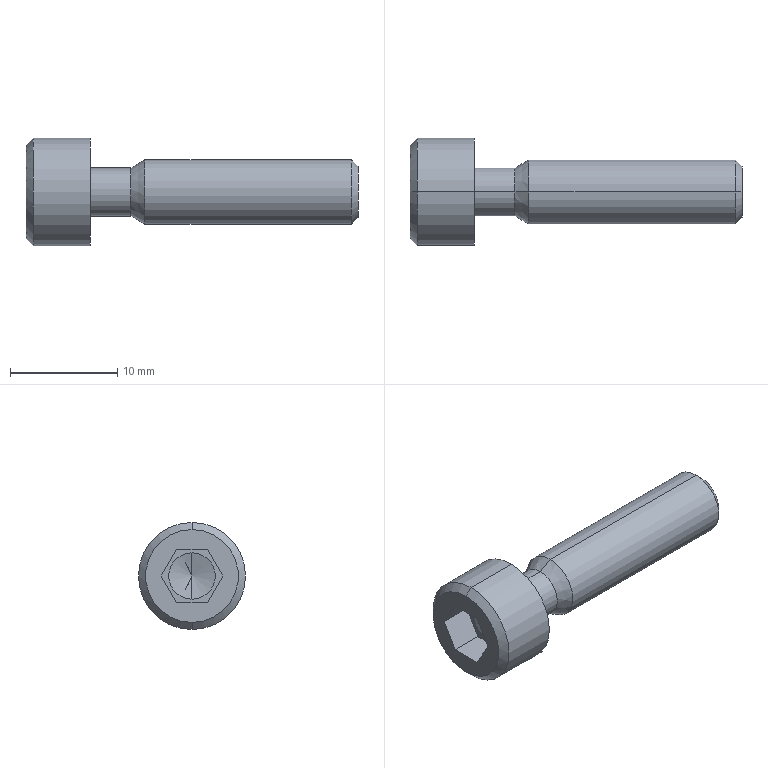Part | STEP file | 0244_Z_019_SCBZ6-25_1 | 1 solid | 24 faces | box 31 x 10 x 10 mm | volume 1045 mm3 | plane 10 | cone 8 | cylinder 6 | commonest cylinder face diameters 4.5 x2 6 x2 10 x2
STEP:
#1=CARTESIAN_POINT('',(0.,0.,0.));
#2=DIRECTION('',(0.,0.,1.));
#3=DIRECTION('',(1.,0.,0.));
#4=AXIS2_PLACEMENT_3D('',#1,#2,#3);
#5=CARTESIAN_POINT('',(5.1,0.,-3.));
#6=VERTEX_POINT('',#5);
#7=CARTESIAN_POINT('',(5.1,0.,3.));
#8=VERTEX_POINT('',#7);
#9=CARTESIAN_POINT('',(5.1,0.,0.));
#10=DIRECTION('',(1.,0.,0.));
#11=DIRECTION('',(0.,0.,-1.));
#12=AXIS2_PLACEMENT_3D('',#9,#10,#11);
#13=CIRCLE('',#12,3.);
#14=CARTESIAN_POINT('',(14.743,0.,0.));
#15=DIRECTION('',(1.,0.,0.));
#16=DIRECTION('',(0.,0.,-1.));
#17=AXIS2_PLACEMENT_3D('',#14,#15,#16);
#18=CYLINDRICAL_SURFACE('',#17,3.);
#19=CARTESIAN_POINT('',(0.,-9.643));
#20=DIRECTION('',(1.,0.));
#21=VECTOR('',#20,1.);
#22=LINE('',#19,#21);
#23=(GEOMETRIC_REPRESENTATION_CONTEXT(2)PARAMETRIC_REPRESENTATION_CONTEXT()REPRESENTATION_CONTEXT('',''));
#24=DEFINITIONAL_REPRESENTATION('',(#22),#23);
#25=PCURVE('',#18,#24);
#26=CARTESIAN_POINT('',(5.1,0.,0.));
#27=DIRECTION('',(1.,0.,0.));
#28=DIRECTION('',(0.,0.,-1.));
#29=AXIS2_PLACEMENT_3D('',#26,#27,#28);
#30=CONICAL_SURFACE('',#29,3.,0.5236);
#31=CARTESIAN_POINT('',(0.,0.));
#32=DIRECTION('',(1.,0.));
#33=VECTOR('',#32,1.);
#34=LINE('',#31,#33);
#35=(GEOMETRIC_REPRESENTATION_CONTEXT(2)PARAMETRIC_REPRESENTATION_CONTEXT()REPRESENTATION_CONTEXT('',''));
#36=DEFINITIONAL_REPRESENTATION('',(#34),#35);
#37=PCURVE('',#30,#36);
#38=SURFACE_CURVE('',#13,(#25,#37),.PCURVE_S1.);
#39=EDGE_CURVE('',#6,#8,#38,.T.);
#40=ORIENTED_EDGE('',*,*,#39,.T.);
#41=CARTESIAN_POINT('',(24.387,0.,3.));
#42=VERTEX_POINT('',#41);
#43=CARTESIAN_POINT('',(14.743,0.,3.));
#44=DIRECTION('',(1.,0.,0.));
#45=VECTOR('',#44,1.);
#46=LINE('',#43,#45);
#47=CARTESIAN_POINT('',(3.142,0.));
#48=DIRECTION('',(0.,1.));
#49=VECTOR('',#48,1.);
#50=LINE('',#47,#49);
#51=(GEOMETRIC_REPRESENTATION_CONTEXT(2)PARAMETRIC_REPRESENTATION_CONTEXT()REPRESENTATION_CONTEXT('',''));
#52=DEFINITIONAL_REPRESENTATION('',(#50),#51);
#53=PCURVE('',#18,#52);
#54=CARTESIAN_POINT('',(14.743,0.,0.));
#55=DIRECTION('',(1.,0.,0.));
#56=DIRECTION('',(0.,0.,-1.));
#57=AXIS2_PLACEMENT_3D('',#54,#55,#56);
#58=CYLINDRICAL_SURFACE('',#57,3.);
#59=CARTESIAN_POINT('',(3.142,0.));
#60=DIRECTION('',(0.,1.));
#61=VECTOR('',#60,1.);
#62=LINE('',#59,#61);
#63=(GEOMETRIC_REPRESENTATION_CONTEXT(2)PARAMETRIC_REPRESENTATION_CONTEXT()REPRESENTATION_CONTEXT('',''));
#64=DEFINITIONAL_REPRESENTATION('',(#62),#63);
#65=PCURVE('',#58,#64);
#66=SURFACE_CURVE('',#46,(#53,#65),.PCURVE_S1.);
#67=EDGE_CURVE('',#8,#42,#66,.T.);
#68=ORIENTED_EDGE('',*,*,#67,.T.);
#69=CARTESIAN_POINT('',(24.387,0.,-3.));
#70=VERTEX_POINT('',#69);
#71=CARTESIAN_POINT('',(24.387,0.,0.));
#72=DIRECTION('',(-1.,0.,0.));
#73=DIRECTION('',(0.,0.,-1.));
#74=AXIS2_PLACEMENT_3D('',#71,#72,#73);
#75=CIRCLE('',#74,3.);
#76=CARTESIAN_POINT('',(6.283,9.643));
#77=DIRECTION('',(-1.,0.));
#78=VECTOR('',#77,1.);
#79=LINE('',#76,#78);
#80=(GEOMETRIC_REPRESENTATION_CONTEXT(2)PARAMETRIC_REPRESENTATION_CONTEXT()REPRESENTATION_CONTEXT('',''));
#81=DEFINITIONAL_REPRESENTATION('',(#79),#80);
#82=PCURVE('',#18,#81);
#83=CARTESIAN_POINT('',(24.386,0.,0.));
#84=DIRECTION('',(-1.,0.,0.));
#85=DIRECTION('',(0.,0.,1.));
#86=AXIS2_PLACEMENT_3D('',#83,#84,#85);
#87=CONICAL_SURFACE('',#86,3.,0.7854);
#88=CARTESIAN_POINT('',(-3.142,0.));
#89=DIRECTION('',(1.,0.));
#90=VECTOR('',#89,1.);
#91=LINE('',#88,#90);
#92=(GEOMETRIC_REPRESENTATION_CONTEXT(2)PARAMETRIC_REPRESENTATION_CONTEXT()REPRESENTATION_CONTEXT('',''));
#93=DEFINITIONAL_REPRESENTATION('',(#91),#92);
#94=PCURVE('',#87,#93);
#95=SURFACE_CURVE('',#75,(#82,#94),.PCURVE_S1.);
#96=EDGE_CURVE('',#42,#70,#95,.T.);
#97=ORIENTED_EDGE('',*,*,#96,.T.);
#98=CARTESIAN_POINT('',(14.743,0.,-3.));
#99=DIRECTION('',(1.,0.,0.));
#100=VECTOR('',#99,1.);
#101=LINE('',#98,#100);
#102=CARTESIAN_POINT('',(0.,0.));
#103=DIRECTION('',(0.,1.));
#104=VECTOR('',#103,1.);
#105=LINE('',#102,#104);
#106=(GEOMETRIC_REPRESENTATION_CONTEXT(2)PARAMETRIC_REPRESENTATION_CONTEXT()REPRESENTATION_CONTEXT('',''));
#107=DEFINITIONAL_REPRESENTATION('',(#105),#106);
#108=PCURVE('',#18,#107);
#109=CARTESIAN_POINT('',(6.283,0.));
#110=DIRECTION('',(0.,1.));
#111=VECTOR('',#110,1.);
#112=LINE('',#109,#111);
#113=(GEOMETRIC_REPRESENTATION_CONTEXT(2)PARAMETRIC_REPRESENTATION_CONTEXT()REPRESENTATION_CONTEXT('',''));
#114=DEFINITIONAL_REPRESENTATION('',(#112),#113);
#115=PCURVE('',#58,#114);
#116=SURFACE_CURVE('',#101,(#108,#115),.PCURVE_S1.);
#117=EDGE_CURVE('',#6,#70,#116,.T.);
#118=ORIENTED_EDGE('',*,*,#117,.F.);
#119=EDGE_LOOP('',(#40,#68,#97,#118));
#120=FACE_BOUND('',#119,.T.);
#121=ADVANCED_FACE('',(#120),#18,.T.);
#122=CARTESIAN_POINT('',(3.801,0.,-2.25));
#123=VERTEX_POINT('',#122);
#124=CARTESIAN_POINT('',(3.801,0.,2.25));
#125=VERTEX_POINT('',#124);
#126=CARTESIAN_POINT('',(3.801,0.,0.));
#127=DIRECTION('',(1.,0.,0.));
#128=DIRECTION('',(0.,1.,0.));
#129=AXIS2_PLACEMENT_3D('',#126,#127,#128);
#130=CIRCLE('',#129,2.25);
#131=CARTESIAN_POINT('',(-4.712,-1.299));
#132=DIRECTION('',(1.,0.));
#133=VECTOR('',#132,1.);
#134=LINE('',#131,#133);
#135=(GEOMETRIC_REPRESENTATION_CONTEXT(2)PARAMETRIC_REPRESENTATION_CONTEXT()REPRESENTATION_CONTEXT('',''));
#136=DEFINITIONAL_REPRESENTATION('',(#134),#135);
#137=PCURVE('',#30,#136);
#138=CARTESIAN_POINT('',(1.9,0.,0.));
#139=DIRECTION('',(1.,0.,0.));
#140=DIRECTION('',(0.,0.,-1.));
#141=AXIS2_PLACEMENT_3D('',#138,#139,#140);
#142=CYLINDRICAL_SURFACE('',#141,2.25);
#143=CARTESIAN_POINT('',(-4.712,1.9));
#144=DIRECTION('',(1.,0.));
#145=VECTOR('',#144,1.);
#146=LINE('',#143,#145);
#147=(GEOMETRIC_REPRESENTATION_CONTEXT(2)PARAMETRIC_REPRESENTATION_CONTEXT()REPRESENTATION_CONTEXT('',''));
#148=DEFINITIONAL_REPRESENTATION('',(#146),#147);
#149=PCURVE('',#142,#148);
#150=SURFACE_CURVE('',#130,(#137,#149),.PCURVE_S1.);
#151=EDGE_CURVE('',#123,#125,#150,.T.);
#152=ORIENTED_EDGE('',*,*,#151,.T.);
#153=CARTESIAN_POINT('',(5.1,0.,3.));
#154=DIRECTION('',(0.866,0.,0.5));
#155=VECTOR('',#154,1.);
#156=LINE('',#153,#155);
#157=CARTESIAN_POINT('',(3.142,0.));
#158=DIRECTION('',(0.,1.));
#159=VECTOR('',#158,1.);
#160=LINE('',#157,#159);
#161=(GEOMETRIC_REPRESENTATION_CONTEXT(2)PARAMETRIC_REPRESENTATION_CONTEXT()REPRESENTATION_CONTEXT('',''));
#162=DEFINITIONAL_REPRESENTATION('',(#160),#161);
#163=PCURVE('',#30,#162);
#164=CARTESIAN_POINT('',(5.1,0.,0.));
#165=DIRECTION('',(1.,0.,0.));
#166=DIRECTION('',(0.,0.,-1.));
#167=AXIS2_PLACEMENT_3D('',#164,#165,#166);
#168=CONICAL_SURFACE('',#167,3.,0.5236);
#169=CARTESIAN_POINT('',(3.142,0.));
#170=DIRECTION('',(0.,1.));
#171=VECTOR('',#170,1.);
#172=LINE('',#169,#171);
#173=(GEOMETRIC_REPRESENTATION_CONTEXT(2)PARAMETRIC_REPRESENTATION_CONTEXT()REPRESENTATION_CONTEXT('',''));
#174=DEFINITIONAL_REPRESENTATION('',(#172),#173);
#175=PCURVE('',#168,#174);
#176=SURFACE_CURVE('',#156,(#163,#175),.PCURVE_S1.);
#177=EDGE_CURVE('',#125,#8,#176,.T.);
#178=ORIENTED_EDGE('',*,*,#177,.T.);
#179=ORIENTED_EDGE('',*,*,#39,.F.);
#180=CARTESIAN_POINT('',(5.1,0.,-3.));
#181=DIRECTION('',(0.866,0.,-0.5));
#182=VECTOR('',#181,1.);
#183=LINE('',#180,#182);
#184=CARTESIAN_POINT('',(0.,0.));
#185=DIRECTION('',(0.,1.));
#186=VECTOR('',#185,1.);
#187=LINE('',#184,#186);
#188=(GEOMETRIC_REPRESENTATION_CONTEXT(2)PARAMETRIC_REPRESENTATION_CONTEXT()REPRESENTATION_CONTEXT('',''));
#189=DEFINITIONAL_REPRESENTATION('',(#187),#188);
#190=PCURVE('',#30,#189);
#191=CARTESIAN_POINT('',(6.283,0.));
#192=DIRECTION('',(0.,1.));
#193=VECTOR('',#192,1.);
#194=LINE('',#191,#193);
#195=(GEOMETRIC_REPRESENTATION_CONTEXT(2)PARAMETRIC_REPRESENTATION_CONTEXT()REPRESENTATION_CONTEXT('',''));
#196=DEFINITIONAL_REPRESENTATION('',(#194),#195);
#197=PCURVE('',#168,#196);
#198=SURFACE_CURVE('',#183,(#190,#197),.PCURVE_S1.);
#199=EDGE_CURVE('',#123,#6,#198,.T.);
#200=ORIENTED_EDGE('',*,*,#199,.F.);
#201=EDGE_LOOP('',(#152,#178,#179,#200));
#202=FACE_BOUND('',#201,.T.);
#203=ADVANCED_FACE('',(#202),#30,.T.);
#204=CARTESIAN_POINT('',(25.,0.,2.386));
#205=VERTEX_POINT('',#204);
#206=CARTESIAN_POINT('',(25.,0.,-2.386));
#207=VERTEX_POINT('',#206);
#208=CARTESIAN_POINT('',(25.,0.,0.));
#209=DIRECTION('',(-1.,0.,0.));
#210=DIRECTION('',(0.,0.,1.));
#211=AXIS2_PLACEMENT_3D('',#208,#209,#210);
#212=CIRCLE('',#211,2.386);
#213=CARTESIAN_POINT('',(0.,-0.6135));
#214=DIRECTION('',(1.,0.));
#215=VECTOR('',#214,1.);
#216=LINE('',#213,#215);
#217=(GEOMETRIC_REPRESENTATION_CONTEXT(2)PARAMETRIC_REPRESENTATION_CONTEXT()REPRESENTATION_CONTEXT('',''));
#218=DEFINITIONAL_REPRESENTATION('',(#216),#217);
#219=PCURVE('',#87,#218);
#220=CARTESIAN_POINT('',(25.,1.193,0.));
#221=DIRECTION('',(1.,0.,0.));
#222=DIRECTION('',(0.,0.,-1.));
#223=AXIS2_PLACEMENT_3D('',#220,#221,#222);
#224=PLANE('',#223);
#225=CARTESIAN_POINT('',(-2.386,-1.193));
#226=CARTESIAN_POINT('',(-2.386,2.94));
#227=CARTESIAN_POINT('',(1.193,0.8735));
#228=CARTESIAN_POINT('',(4.773,-1.193));
#229=CARTESIAN_POINT('',(1.193,-3.26));
#230=CARTESIAN_POINT('',(-2.386,-5.327));
#231=CARTESIAN_POINT('',(-2.386,-1.193));
#232=(BOUNDED_CURVE()B_SPLINE_CURVE(2,(#225,#226,#227,#228,#229,#230,#231),.UNSPECIFIED.,.T.,.F.)B_SPLINE_CURVE_WITH_KNOTS((1,2,2,2,2,1),(-2.094,0.,2.094,4.189,6.283,8.378),.UNSPECIFIED.)CURVE()GEOMETRIC_REPRESENTATION_ITEM()RATIONAL_B_SPLINE_CURVE((1.,0.5,1.,0.5,1.,0.5,1.))REPRESENTATION_ITEM(''));
#233=(GEOMETRIC_REPRESENTATION_CONTEXT(2)PARAMETRIC_REPRESENTATION_CONTEXT()REPRESENTATION_CONTEXT('',''));
#234=DEFINITIONAL_REPRESENTATION('',(#232),#233);
#235=PCURVE('',#224,#234);
#236=SURFACE_CURVE('',#212,(#219,#235),.PCURVE_S1.);
#237=EDGE_CURVE('',#205,#207,#236,.T.);
#238=ORIENTED_EDGE('',*,*,#237,.T.);
#239=CARTESIAN_POINT('',(24.386,0.,-3.));
#240=DIRECTION('',(-0.7071,0.,-0.7071));
#241=VECTOR('',#240,1.);
#242=LINE('',#239,#241);
#243=CARTESIAN_POINT('',(3.142,0.));
#244=DIRECTION('',(0.,1.));
#245=VECTOR('',#244,1.);
#246=LINE('',#243,#245);
#247=(GEOMETRIC_REPRESENTATION_CONTEXT(2)PARAMETRIC_REPRESENTATION_CONTEXT()REPRESENTATION_CONTEXT('',''));
#248=DEFINITIONAL_REPRESENTATION('',(#246),#247);
#249=PCURVE('',#87,#248);
#250=CARTESIAN_POINT('',(24.386,0.,0.));
#251=DIRECTION('',(-1.,0.,0.));
#252=DIRECTION('',(0.,0.,1.));
#253=AXIS2_PLACEMENT_3D('',#250,#251,#252);
#254=CONICAL_SURFACE('',#253,3.,0.7854);
#255=CARTESIAN_POINT('',(3.142,0.));
#256=DIRECTION('',(0.,1.));
#257=VECTOR('',#256,1.);
#258=LINE('',#255,#257);
#259=(GEOMETRIC_REPRESENTATION_CONTEXT(2)PARAMETRIC_REPRESENTATION_CONTEXT()REPRESENTATION_CONTEXT('',''));
#260=DEFINITIONAL_REPRESENTATION('',(#258),#259);
#261=PCURVE('',#254,#260);
#262=SURFACE_CURVE('',#242,(#249,#261),.PCURVE_S1.);
#263=EDGE_CURVE('',#207,#70,#262,.T.);
#264=ORIENTED_EDGE('',*,*,#263,.T.);
#265=ORIENTED_EDGE('',*,*,#96,.F.);
#266=CARTESIAN_POINT('',(24.386,0.,3.));
#267=DIRECTION('',(-0.7071,0.,0.7071));
#268=VECTOR('',#267,1.);
#269=LINE('',#266,#268);
#270=CARTESIAN_POINT('',(0.,0.));
#271=DIRECTION('',(0.,1.));
#272=VECTOR('',#271,1.);
#273=LINE('',#270,#272);
#274=(GEOMETRIC_REPRESENTATION_CONTEXT(2)PARAMETRIC_REPRESENTATION_CONTEXT()REPRESENTATION_CONTEXT('',''));
#275=DEFINITIONAL_REPRESENTATION('',(#273),#274);
#276=PCURVE('',#87,#275);
#277=CARTESIAN_POINT('',(6.283,0.));
#278=DIRECTION('',(0.,1.));
#279=VECTOR('',#278,1.);
#280=LINE('',#277,#279);
#281=(GEOMETRIC_REPRESENTATION_CONTEXT(2)PARAMETRIC_REPRESENTATION_CONTEXT()REPRESENTATION_CONTEXT('',''));
#282=DEFINITIONAL_REPRESENTATION('',(#280),#281);
#283=PCURVE('',#254,#282);
#284=SURFACE_CURVE('',#269,(#276,#283),.PCURVE_S1.);
#285=EDGE_CURVE('',#205,#42,#284,.T.);
#286=ORIENTED_EDGE('',*,*,#285,.F.);
#287=EDGE_LOOP('',(#238,#264,#265,#286));
#288=FACE_BOUND('',#287,.T.);
#289=ADVANCED_FACE('',(#288),#87,.T.);
#290=CARTESIAN_POINT('',(0.,0.,-2.25));
#291=VERTEX_POINT('',#290);
#292=CARTESIAN_POINT('',(0.,0.,2.25));
#293=VERTEX_POINT('',#292);
#294=CARTESIAN_POINT('',(0.,0.,0.));
#295=DIRECTION('',(1.,0.,0.));
#296=DIRECTION('',(0.,0.,-1.));
#297=AXIS2_PLACEMENT_3D('',#294,#295,#296);
#298=CIRCLE('',#297,2.25);
#299=CARTESIAN_POINT('',(0.,-1.9));
#300=DIRECTION('',(1.,0.));
#301=VECTOR('',#300,1.);
#302=LINE('',#299,#301);
#303=(GEOMETRIC_REPRESENTATION_CONTEXT(2)PARAMETRIC_REPRESENTATION_CONTEXT()REPRESENTATION_CONTEXT('',''));
#304=DEFINITIONAL_REPRESENTATION('',(#302),#303);
#305=PCURVE('',#142,#304);
#306=CARTESIAN_POINT('',(0.,3.625,0.));
#307=DIRECTION('',(1.,0.,0.));
#308=DIRECTION('',(0.,0.,-1.));
#309=AXIS2_PLACEMENT_3D('',#306,#307,#308);
#310=PLANE('',#309);
#311=CARTESIAN_POINT('',(0.,-3.625));
#312=DIRECTION('',(1.,0.));
#313=AXIS2_PLACEMENT_2D('',#311,#312);
#314=CIRCLE('',#313,2.25);
#315=(GEOMETRIC_REPRESENTATION_CONTEXT(2)PARAMETRIC_REPRESENTATION_CONTEXT()REPRESENTATION_CONTEXT('',''));
#316=DEFINITIONAL_REPRESENTATION('',(#314),#315);
#317=PCURVE('',#310,#316);
#318=SURFACE_CURVE('',#298,(#305,#317),.PCURVE_S1.);
#319=EDGE_CURVE('',#291,#293,#318,.T.);
#320=ORIENTED_EDGE('',*,*,#319,.T.);
#321=CARTESIAN_POINT('',(1.9,0.,2.25));
#322=DIRECTION('',(1.,0.,0.));
#323=VECTOR('',#322,1.);
#324=LINE('',#321,#323);
#325=CARTESIAN_POINT('',(3.142,0.));
#326=DIRECTION('',(0.,1.));
#327=VECTOR('',#326,1.);
#328=LINE('',#325,#327);
#329=(GEOMETRIC_REPRESENTATION_CONTEXT(2)PARAMETRIC_REPRESENTATION_CONTEXT()REPRESENTATION_CONTEXT('',''));
#330=DEFINITIONAL_REPRESENTATION('',(#328),#329);
#331=PCURVE('',#142,#330);
#332=CARTESIAN_POINT('',(1.9,0.,0.));
#333=DIRECTION('',(1.,0.,0.));
#334=DIRECTION('',(0.,0.,-1.));
#335=AXIS2_PLACEMENT_3D('',#332,#333,#334);
#336=CYLINDRICAL_SURFACE('',#335,2.25);
#337=CARTESIAN_POINT('',(3.142,0.));
#338=DIRECTION('',(0.,1.));
#339=VECTOR('',#338,1.);
#340=LINE('',#337,#339);
#341=(GEOMETRIC_REPRESENTATION_CONTEXT(2)PARAMETRIC_REPRESENTATION_CONTEXT()REPRESENTATION_CONTEXT('',''));
#342=DEFINITIONAL_REPRESENTATION('',(#340),#341);
#343=PCURVE('',#336,#342);
#344=SURFACE_CURVE('',#324,(#331,#343),.PCURVE_S1.);
#345=EDGE_CURVE('',#293,#125,#344,.T.);
#346=ORIENTED_EDGE('',*,*,#345,.T.);
#347=ORIENTED_EDGE('',*,*,#151,.F.);
#348=CARTESIAN_POINT('',(1.9,0.,-2.25));
#349=DIRECTION('',(1.,0.,0.));
#350=VECTOR('',#349,1.);
#351=LINE('',#348,#350);
#352=CARTESIAN_POINT('',(0.,0.));
#353=DIRECTION('',(0.,1.));
#354=VECTOR('',#353,1.);
#355=LINE('',#352,#354);
#356=(GEOMETRIC_REPRESENTATION_CONTEXT(2)PARAMETRIC_REPRESENTATION_CONTEXT()REPRESENTATION_CONTEXT('',''));
#357=DEFINITIONAL_REPRESENTATION('',(#355),#356);
#358=PCURVE('',#142,#357);
#359=CARTESIAN_POINT('',(6.283,0.));
#360=DIRECTION('',(0.,1.));
#361=VECTOR('',#360,1.);
#362=LINE('',#359,#361);
#363=(GEOMETRIC_REPRESENTATION_CONTEXT(2)PARAMETRIC_REPRESENTATION_CONTEXT()REPRESENTATION_CONTEXT('',''));
#364=DEFINITIONAL_REPRESENTATION('',(#362),#363);
#365=PCURVE('',#336,#364);
#366=SURFACE_CURVE('',#351,(#358,#365),.PCURVE_S1.);
#367=EDGE_CURVE('',#291,#123,#366,.T.);
#368=ORIENTED_EDGE('',*,*,#367,.F.);
#369=EDGE_LOOP('',(#320,#346,#347,#368));
#370=FACE_BOUND('',#369,.T.);
#371=ADVANCED_FACE('',(#370),#142,.T.);
#372=CARTESIAN_POINT('',(-5.333,0.,-5.));
#373=VERTEX_POINT('',#372);
#374=CARTESIAN_POINT('',(-5.333,0.,5.));
#375=VERTEX_POINT('',#374);
#376=CARTESIAN_POINT('',(-5.333,0.,0.));
#377=DIRECTION('',(1.,0.,0.));
#378=DIRECTION('',(0.,0.,-1.));
#379=AXIS2_PLACEMENT_3D('',#376,#377,#378);
#380=CIRCLE('',#379,5.);
#381=CARTESIAN_POINT('',(-2.667,0.,0.));
#382=DIRECTION('',(1.,0.,0.));
#383=DIRECTION('',(0.,0.,-1.));
#384=AXIS2_PLACEMENT_3D('',#381,#382,#383);
#385=CYLINDRICAL_SURFACE('',#384,5.);
#386=CARTESIAN_POINT('',(0.,-2.667));
#387=DIRECTION('',(1.,0.));
#388=VECTOR('',#387,1.);
#389=LINE('',#386,#388);
#390=(GEOMETRIC_REPRESENTATION_CONTEXT(2)PARAMETRIC_REPRESENTATION_CONTEXT()REPRESENTATION_CONTEXT('',''));
#391=DEFINITIONAL_REPRESENTATION('',(#389),#390);
#392=PCURVE('',#385,#391);
#393=CARTESIAN_POINT('',(-5.333,0.,0.));
#394=DIRECTION('',(1.,0.,0.));
#395=DIRECTION('',(0.,0.,-1.));
#396=AXIS2_PLACEMENT_3D('',#393,#394,#395);
#397=CONICAL_SURFACE('',#396,5.,0.7854);
#398=CARTESIAN_POINT('',(0.,0.));
#399=DIRECTION('',(1.,0.));
#400=VECTOR('',#399,1.);
#401=LINE('',#398,#400);
#402=(GEOMETRIC_REPRESENTATION_CONTEXT(2)PARAMETRIC_REPRESENTATION_CONTEXT()REPRESENTATION_CONTEXT('',''));
#403=DEFINITIONAL_REPRESENTATION('',(#401),#402);
#404=PCURVE('',#397,#403);
#405=SURFACE_CURVE('',#380,(#392,#404),.PCURVE_S1.);
#406=EDGE_CURVE('',#373,#375,#405,.T.);
#407=ORIENTED_EDGE('',*,*,#406,.T.);
#408=CARTESIAN_POINT('',(0.,0.,5.));
#409=VERTEX_POINT('',#408);
#410=CARTESIAN_POINT('',(-2.667,0.,5.));
#411=DIRECTION('',(1.,0.,0.));
#412=VECTOR('',#411,1.);
#413=LINE('',#410,#412);
#414=CARTESIAN_POINT('',(3.142,0.));
#415=DIRECTION('',(0.,1.));
#416=VECTOR('',#415,1.);
#417=LINE('',#414,#416);
#418=(GEOMETRIC_REPRESENTATION_CONTEXT(2)PARAMETRIC_REPRESENTATION_CONTEXT()REPRESENTATION_CONTEXT('',''));
#419=DEFINITIONAL_REPRESENTATION('',(#417),#418);
#420=PCURVE('',#385,#419);
#421=CARTESIAN_POINT('',(-2.667,0.,0.));
#422=DIRECTION('',(1.,0.,0.));
#423=DIRECTION('',(0.,0.,-1.));
#424=AXIS2_PLACEMENT_3D('',#421,#422,#423);
#425=CYLINDRICAL_SURFACE('',#424,5.);
#426=CARTESIAN_POINT('',(3.142,0.));
#427=DIRECTION('',(0.,1.));
#428=VECTOR('',#427,1.);
#429=LINE('',#426,#428);
#430=(GEOMETRIC_REPRESENTATION_CONTEXT(2)PARAMETRIC_REPRESENTATION_CONTEXT()REPRESENTATION_CONTEXT('',''));
#431=DEFINITIONAL_REPRESENTATION('',(#429),#430);
#432=PCURVE('',#425,#431);
#433=SURFACE_CURVE('',#413,(#420,#432),.PCURVE_S1.);
#434=EDGE_CURVE('',#375,#409,#433,.T.);
#435=ORIENTED_EDGE('',*,*,#434,.T.);
#436=CARTESIAN_POINT('',(0.,0.,-5.));
#437=VERTEX_POINT('',#436);
#438=CARTESIAN_POINT('',(0.,0.,0.));
#439=DIRECTION('',(1.,0.,0.));
#440=DIRECTION('',(0.,0.,-1.));
#441=AXIS2_PLACEMENT_3D('',#438,#439,#440);
#442=CIRCLE('',#441,5.);
#443=CARTESIAN_POINT('',(0.,2.667));
#444=DIRECTION('',(1.,0.));
#445=VECTOR('',#444,1.);
#446=LINE('',#443,#445);
#447=(GEOMETRIC_REPRESENTATION_CONTEXT(2)PARAMETRIC_REPRESENTATION_CONTEXT()REPRESENTATION_CONTEXT('',''));
#448=DEFINITIONAL_REPRESENTATION('',(#446),#447);
#449=PCURVE('',#385,#448);
#450=CARTESIAN_POINT('',(0.,-3.625));
#451=DIRECTION('',(1.,0.));
#452=AXIS2_PLACEMENT_2D('',#450,#451);
#453=CIRCLE('',#452,5.);
#454=(GEOMETRIC_REPRESENTATION_CONTEXT(2)PARAMETRIC_REPRESENTATION_CONTEXT()REPRESENTATION_CONTEXT('',''));
#455=DEFINITIONAL_REPRESENTATION('',(#453),#454);
#456=PCURVE('',#310,#455);
#457=SURFACE_CURVE('',#442,(#449,#456),.PCURVE_S1.);
#458=EDGE_CURVE('',#437,#409,#457,.T.);
#459=ORIENTED_EDGE('',*,*,#458,.F.);
#460=CARTESIAN_POINT('',(-2.667,0.,-5.));
#461=DIRECTION('',(1.,0.,0.));
#462=VECTOR('',#461,1.);
#463=LINE('',#460,#462);
#464=CARTESIAN_POINT('',(0.,0.));
#465=DIRECTION('',(0.,1.));
#466=VECTOR('',#465,1.);
#467=LINE('',#464,#466);
#468=(GEOMETRIC_REPRESENTATION_CONTEXT(2)PARAMETRIC_REPRESENTATION_CONTEXT()REPRESENTATION_CONTEXT('',''));
#469=DEFINITIONAL_REPRESENTATION('',(#467),#468);
#470=PCURVE('',#385,#469);
#471=CARTESIAN_POINT('',(6.283,0.));
#472=DIRECTION('',(0.,1.));
#473=VECTOR('',#472,1.);
#474=LINE('',#471,#473);
#475=(GEOMETRIC_REPRESENTATION_CONTEXT(2)PARAMETRIC_REPRESENTATION_CONTEXT()REPRESENTATION_CONTEXT('',''));
#476=DEFINITIONAL_REPRESENTATION('',(#474),#475);
#477=PCURVE('',#425,#476);
#478=SURFACE_CURVE('',#463,(#470,#477),.PCURVE_S1.);
#479=EDGE_CURVE('',#373,#437,#478,.T.);
#480=ORIENTED_EDGE('',*,*,#479,.F.);
#481=EDGE_LOOP('',(#407,#435,#459,#480));
#482=FACE_BOUND('',#481,.T.);
#483=ADVANCED_FACE('',(#482),#385,.T.);
#484=CARTESIAN_POINT('',(-6.,0.,-4.333));
#485=VERTEX_POINT('',#484);
#486=CARTESIAN_POINT('',(-6.,0.,4.333));
#487=VERTEX_POINT('',#486);
#488=CARTESIAN_POINT('',(-6.,0.,0.));
#489=DIRECTION('',(1.,0.,0.));
#490=DIRECTION('',(0.,0.,-1.));
#491=AXIS2_PLACEMENT_3D('',#488,#489,#490);
#492=CIRCLE('',#491,4.333);
#493=CARTESIAN_POINT('',(0.,-0.6667));
#494=DIRECTION('',(1.,0.));
#495=VECTOR('',#494,1.);
#496=LINE('',#493,#495);
#497=(GEOMETRIC_REPRESENTATION_CONTEXT(2)PARAMETRIC_REPRESENTATION_CONTEXT()REPRESENTATION_CONTEXT('',''));
#498=DEFINITIONAL_REPRESENTATION('',(#496),#497);
#499=PCURVE('',#397,#498);
#500=CARTESIAN_POINT('',(-6.,3.417,0.));
#501=DIRECTION('',(-1.,0.,0.));
#502=DIRECTION('',(0.,0.,1.));
#503=AXIS2_PLACEMENT_3D('',#500,#501,#502);
#504=PLANE('',#503);
#505=CARTESIAN_POINT('',(-4.333,-3.417));
#506=CARTESIAN_POINT('',(-4.333,4.089));
#507=CARTESIAN_POINT('',(2.167,0.3361));
#508=CARTESIAN_POINT('',(8.667,-3.417));
#509=CARTESIAN_POINT('',(2.167,-7.169));
#510=CARTESIAN_POINT('',(-4.333,-10.922));
#511=CARTESIAN_POINT('',(-4.333,-3.417));
#512=(BOUNDED_CURVE()B_SPLINE_CURVE(2,(#505,#506,#507,#508,#509,#510,#511),.UNSPECIFIED.,.T.,.F.)B_SPLINE_CURVE_WITH_KNOTS((1,2,2,2,2,1),(-2.094,0.,2.094,4.189,6.283,8.378),.UNSPECIFIED.)CURVE()GEOMETRIC_REPRESENTATION_ITEM()RATIONAL_B_SPLINE_CURVE((1.,0.5,1.,0.5,1.,0.5,1.))REPRESENTATION_ITEM(''));
#513=(GEOMETRIC_REPRESENTATION_CONTEXT(2)PARAMETRIC_REPRESENTATION_CONTEXT()REPRESENTATION_CONTEXT('',''));
#514=DEFINITIONAL_REPRESENTATION('',(#512),#513);
#515=PCURVE('',#504,#514);
#516=SURFACE_CURVE('',#492,(#499,#515),.PCURVE_S1.);
#517=EDGE_CURVE('',#485,#487,#516,.T.);
#518=ORIENTED_EDGE('',*,*,#517,.T.);
#519=CARTESIAN_POINT('',(-5.333,0.,5.));
#520=DIRECTION('',(0.7071,0.,0.7071));
#521=VECTOR('',#520,1.);
#522=LINE('',#519,#521);
#523=CARTESIAN_POINT('',(3.142,0.));
#524=DIRECTION('',(0.,1.));
#525=VECTOR('',#524,1.);
#526=LINE('',#523,#525);
#527=(GEOMETRIC_REPRESENTATION_CONTEXT(2)PARAMETRIC_REPRESENTATION_CONTEXT()REPRESENTATION_CONTEXT('',''));
#528=DEFINITIONAL_REPRESENTATION('',(#526),#527);
#529=PCURVE('',#397,#528);
#530=CARTESIAN_POINT('',(-5.333,0.,0.));
#531=DIRECTION('',(1.,0.,0.));
#532=DIRECTION('',(0.,0.,-1.));
#533=AXIS2_PLACEMENT_3D('',#530,#531,#532);
#534=CONICAL_SURFACE('',#533,5.,0.7854);
#535=CARTESIAN_POINT('',(3.142,0.));
#536=DIRECTION('',(0.,1.));
#537=VECTOR('',#536,1.);
#538=LINE('',#535,#537);
#539=(GEOMETRIC_REPRESENTATION_CONTEXT(2)PARAMETRIC_REPRESENTATION_CONTEXT()REPRESENTATION_CONTEXT('',''));
#540=DEFINITIONAL_REPRESENTATION('',(#538),#539);
#541=PCURVE('',#534,#540);
#542=SURFACE_CURVE('',#522,(#529,#541),.PCURVE_S1.);
#543=EDGE_CURVE('',#487,#375,#542,.T.);
#544=ORIENTED_EDGE('',*,*,#543,.T.);
#545=ORIENTED_EDGE('',*,*,#406,.F.);
#546=CARTESIAN_POINT('',(-5.333,0.,-5.));
#547=DIRECTION('',(0.7071,0.,-0.7071));
#548=VECTOR('',#547,1.);
#549=LINE('',#546,#548);
#550=CARTESIAN_POINT('',(0.,0.));
#551=DIRECTION('',(0.,1.));
#552=VECTOR('',#551,1.);
#553=LINE('',#550,#552);
#554=(GEOMETRIC_REPRESENTATION_CONTEXT(2)PARAMETRIC_REPRESENTATION_CONTEXT()REPRESENTATION_CONTEXT('',''));
#555=DEFINITIONAL_REPRESENTATION('',(#553),#554);
#556=PCURVE('',#397,#555);
#557=CARTESIAN_POINT('',(6.283,0.));
#558=DIRECTION('',(0.,1.));
#559=VECTOR('',#558,1.);
#560=LINE('',#557,#559);
#561=(GEOMETRIC_REPRESENTATION_CONTEXT(2)PARAMETRIC_REPRESENTATION_CONTEXT()REPRESENTATION_CONTEXT('',''));
#562=DEFINITIONAL_REPRESENTATION('',(#560),#561);
#563=PCURVE('',#534,#562);
#564=SURFACE_CURVE('',#549,(#556,#563),.PCURVE_S1.);
#565=EDGE_CURVE('',#485,#373,#564,.T.);
#566=ORIENTED_EDGE('',*,*,#565,.F.);
#567=EDGE_LOOP('',(#518,#544,#545,#566));
#568=FACE_BOUND('',#567,.T.);
#569=ADVANCED_FACE('',(#568),#397,.T.);
#570=CARTESIAN_POINT('',(-3.,0.,-2.167));
#571=VERTEX_POINT('',#570);
#572=CARTESIAN_POINT('',(-3.,0.,2.167));
#573=VERTEX_POINT('',#572);
#574=CARTESIAN_POINT('',(-3.,0.,0.));
#575=DIRECTION('',(-1.,0.,0.));
#576=DIRECTION('',(0.,0.,1.));
#577=AXIS2_PLACEMENT_3D('',#574,#575,#576);
#578=CIRCLE('',#577,2.167);
#579=CARTESIAN_POINT('',(-3.,0.,0.));
#580=DIRECTION('',(-1.,0.,0.));
#581=DIRECTION('',(0.,0.,1.));
#582=AXIS2_PLACEMENT_3D('',#579,#580,#581);
#583=CONICAL_SURFACE('',#582,2.167,1.309);
#584=CARTESIAN_POINT('',(0.,0.));
#585=DIRECTION('',(1.,0.));
#586=VECTOR('',#585,1.);
#587=LINE('',#584,#586);
#588=(GEOMETRIC_REPRESENTATION_CONTEXT(2)PARAMETRIC_REPRESENTATION_CONTEXT()REPRESENTATION_CONTEXT('',''));
#589=DEFINITIONAL_REPRESENTATION('',(#587),#588);
#590=PCURVE('',#583,#589);
#591=CARTESIAN_POINT('',(-3.,0.,0.));
#592=DIRECTION('',(1.,0.,0.));
#593=DIRECTION('',(0.,0.,-1.));
#594=AXIS2_PLACEMENT_3D('',#591,#592,#593);
#595=PLANE('',#594);
#596=CARTESIAN_POINT('',(-2.167,0.));
#597=CARTESIAN_POINT('',(-2.167,3.753));
#598=CARTESIAN_POINT('',(1.083,1.876));
#599=CARTESIAN_POINT('',(4.333,0.));
#600=CARTESIAN_POINT('',(1.083,-1.876));
#601=CARTESIAN_POINT('',(-2.167,-3.753));
#602=CARTESIAN_POINT('',(-2.167,0.));
#603=(BOUNDED_CURVE()B_SPLINE_CURVE(2,(#596,#597,#598,#599,#600,#601,#602),.UNSPECIFIED.,.T.,.F.)B_SPLINE_CURVE_WITH_KNOTS((1,2,2,2,2,1),(-2.094,0.,2.094,4.189,6.283,8.378),.UNSPECIFIED.)CURVE()GEOMETRIC_REPRESENTATION_ITEM()RATIONAL_B_SPLINE_CURVE((1.,0.5,1.,0.5,1.,0.5,1.))REPRESENTATION_ITEM(''));
#604=(GEOMETRIC_REPRESENTATION_CONTEXT(2)PARAMETRIC_REPRESENTATION_CONTEXT()REPRESENTATION_CONTEXT('',''));
#605=DEFINITIONAL_REPRESENTATION('',(#603),#604);
#606=PCURVE('',#595,#605);
#607=SURFACE_CURVE('',#578,(#590,#606),.PCURVE_S1.);
#608=EDGE_CURVE('',#571,#573,#607,.T.);
#609=ORIENTED_EDGE('',*,*,#608,.F.);
#610=CARTESIAN_POINT('',(-2.419,0.,0.));
#611=VERTEX_POINT('',#610);
#612=CARTESIAN_POINT('',(-3.,0.,-2.167));
#613=DIRECTION('',(-0.2588,0.,-0.9659));
#614=VECTOR('',#613,1.);
#615=LINE('',#612,#614);
#616=CARTESIAN_POINT('',(3.142,0.));
#617=DIRECTION('',(0.,1.));
#618=VECTOR('',#617,1.);
#619=LINE('',#616,#618);
#620=(GEOMETRIC_REPRESENTATION_CONTEXT(2)PARAMETRIC_REPRESENTATION_CONTEXT()REPRESENTATION_CONTEXT('',''));
#621=DEFINITIONAL_REPRESENTATION('',(#619),#620);
#622=PCURVE('',#583,#621);
#623=CARTESIAN_POINT('',(-3.,0.,0.));
#624=DIRECTION('',(-1.,0.,0.));
#625=DIRECTION('',(0.,0.,1.));
#626=AXIS2_PLACEMENT_3D('',#623,#624,#625);
#627=CONICAL_SURFACE('',#626,2.167,1.309);
#628=CARTESIAN_POINT('',(3.142,0.));
#629=DIRECTION('',(0.,1.));
#630=VECTOR('',#629,1.);
#631=LINE('',#628,#630);
#632=(GEOMETRIC_REPRESENTATION_CONTEXT(2)PARAMETRIC_REPRESENTATION_CONTEXT()REPRESENTATION_CONTEXT('',''));
#633=DEFINITIONAL_REPRESENTATION('',(#631),#632);
#634=PCURVE('',#627,#633);
#635=SURFACE_CURVE('',#615,(#622,#634),.PCURVE_S1.);
#636=EDGE_CURVE('',#611,#571,#635,.T.);
#637=ORIENTED_EDGE('',*,*,#636,.F.);
#638=CARTESIAN_POINT('',(-3.,0.,2.167));
#639=DIRECTION('',(-0.2588,0.,0.9659));
#640=VECTOR('',#639,1.);
#641=LINE('',#638,#640);
#642=CARTESIAN_POINT('',(6.283,0.));
#643=DIRECTION('',(0.,1.));
#644=VECTOR('',#643,1.);
#645=LINE('',#642,#644);
#646=(GEOMETRIC_REPRESENTATION_CONTEXT(2)PARAMETRIC_REPRESENTATION_CONTEXT()REPRESENTATION_CONTEXT('',''));
#647=DEFINITIONAL_REPRESENTATION('',(#645),#646);
#648=PCURVE('',#583,#647);
#649=CARTESIAN_POINT('',(0.,0.));
#650=DIRECTION('',(0.,1.));
#651=VECTOR('',#650,1.);
#652=LINE('',#649,#651);
#653=(GEOMETRIC_REPRESENTATION_CONTEXT(2)PARAMETRIC_REPRESENTATION_CONTEXT()REPRESENTATION_CONTEXT('',''));
#654=DEFINITIONAL_REPRESENTATION('',(#652),#653);
#655=PCURVE('',#627,#654);
#656=SURFACE_CURVE('',#641,(#648,#655),.PCURVE_S1.);
#657=EDGE_CURVE('',#611,#573,#656,.T.);
#658=ORIENTED_EDGE('',*,*,#657,.T.);
#659=EDGE_LOOP('',(#609,#637,#658));
#660=FACE_BOUND('',#659,.F.);
#661=ADVANCED_FACE('',(#660),#583,.F.);
#662=ORIENTED_EDGE('',*,*,#67,.F.);
#663=CARTESIAN_POINT('',(5.1,0.,0.));
#664=DIRECTION('',(1.,0.,0.));
#665=DIRECTION('',(0.,0.,-1.));
#666=AXIS2_PLACEMENT_3D('',#663,#664,#665);
#667=CIRCLE('',#666,3.);
#668=CARTESIAN_POINT('',(0.,-9.643));
#669=DIRECTION('',(1.,0.));
#670=VECTOR('',#669,1.);
#671=LINE('',#668,#670);
#672=(GEOMETRIC_REPRESENTATION_CONTEXT(2)PARAMETRIC_REPRESENTATION_CONTEXT()REPRESENTATION_CONTEXT('',''));
#673=DEFINITIONAL_REPRESENTATION('',(#671),#672);
#674=PCURVE('',#58,#673);
#675=CARTESIAN_POINT('',(0.,0.));
#676=DIRECTION('',(1.,0.));
#677=VECTOR('',#676,1.);
#678=LINE('',#675,#677);
#679=(GEOMETRIC_REPRESENTATION_CONTEXT(2)PARAMETRIC_REPRESENTATION_CONTEXT()REPRESENTATION_CONTEXT('',''));
#680=DEFINITIONAL_REPRESENTATION('',(#678),#679);
#681=PCURVE('',#168,#680);
#682=SURFACE_CURVE('',#667,(#674,#681),.PCURVE_S1.);
#683=EDGE_CURVE('',#8,#6,#682,.T.);
#684=ORIENTED_EDGE('',*,*,#683,.T.);
#685=ORIENTED_EDGE('',*,*,#117,.T.);
#686=CARTESIAN_POINT('',(24.387,0.,0.));
#687=DIRECTION('',(-1.,0.,0.));
#688=DIRECTION('',(0.,0.,-1.));
#689=AXIS2_PLACEMENT_3D('',#686,#687,#688);
#690=CIRCLE('',#689,3.);
#691=CARTESIAN_POINT('',(6.283,9.643));
#692=DIRECTION('',(-1.,0.));
#693=VECTOR('',#692,1.);
#694=LINE('',#691,#693);
#695=(GEOMETRIC_REPRESENTATION_CONTEXT(2)PARAMETRIC_REPRESENTATION_CONTEXT()REPRESENTATION_CONTEXT('',''));
#696=DEFINITIONAL_REPRESENTATION('',(#694),#695);
#697=PCURVE('',#58,#696);
#698=CARTESIAN_POINT('',(3.142,0.));
#699=DIRECTION('',(1.,0.));
#700=VECTOR('',#699,1.);
#701=LINE('',#698,#700);
#702=(GEOMETRIC_REPRESENTATION_CONTEXT(2)PARAMETRIC_REPRESENTATION_CONTEXT()REPRESENTATION_CONTEXT('',''));
#703=DEFINITIONAL_REPRESENTATION('',(#701),#702);
#704=PCURVE('',#254,#703);
#705=SURFACE_CURVE('',#690,(#697,#704),.PCURVE_S1.);
#706=EDGE_CURVE('',#70,#42,#705,.T.);
#707=ORIENTED_EDGE('',*,*,#706,.T.);
#708=EDGE_LOOP('',(#662,#684,#685,#707));
#709=FACE_BOUND('',#708,.T.);
#710=ADVANCED_FACE('',(#709),#58,.T.);
#711=ORIENTED_EDGE('',*,*,#177,.F.);
#712=CARTESIAN_POINT('',(3.801,0.,0.));
#713=DIRECTION('',(1.,0.,0.));
#714=DIRECTION('',(0.,1.,0.));
#715=AXIS2_PLACEMENT_3D('',#712,#713,#714);
#716=CIRCLE('',#715,2.25);
#717=CARTESIAN_POINT('',(1.571,-1.299));
#718=DIRECTION('',(1.,0.));
#719=VECTOR('',#718,1.);
#720=LINE('',#717,#719);
#721=(GEOMETRIC_REPRESENTATION_CONTEXT(2)PARAMETRIC_REPRESENTATION_CONTEXT()REPRESENTATION_CONTEXT('',''));
#722=DEFINITIONAL_REPRESENTATION('',(#720),#721);
#723=PCURVE('',#168,#722);
#724=CARTESIAN_POINT('',(1.571,1.9));
#725=DIRECTION('',(1.,0.));
#726=VECTOR('',#725,1.);
#727=LINE('',#724,#726);
#728=(GEOMETRIC_REPRESENTATION_CONTEXT(2)PARAMETRIC_REPRESENTATION_CONTEXT()REPRESENTATION_CONTEXT('',''));
#729=DEFINITIONAL_REPRESENTATION('',(#727),#728);
#730=PCURVE('',#336,#729);
#731=SURFACE_CURVE('',#716,(#723,#730),.PCURVE_S1.);
#732=EDGE_CURVE('',#125,#123,#731,.T.);
#733=ORIENTED_EDGE('',*,*,#732,.T.);
#734=ORIENTED_EDGE('',*,*,#199,.T.);
#735=ORIENTED_EDGE('',*,*,#683,.F.);
#736=EDGE_LOOP('',(#711,#733,#734,#735));
#737=FACE_BOUND('',#736,.T.);
#738=ADVANCED_FACE('',(#737),#168,.T.);
#739=ORIENTED_EDGE('',*,*,#263,.F.);
#740=CARTESIAN_POINT('',(25.,0.,0.));
#741=DIRECTION('',(-1.,0.,0.));
#742=DIRECTION('',(0.,0.,1.));
#743=AXIS2_PLACEMENT_3D('',#740,#741,#742);
#744=CIRCLE('',#743,2.386);
#745=CARTESIAN_POINT('',(0.,-0.6135));
#746=DIRECTION('',(1.,0.));
#747=VECTOR('',#746,1.);
#748=LINE('',#745,#747);
#749=(GEOMETRIC_REPRESENTATION_CONTEXT(2)PARAMETRIC_REPRESENTATION_CONTEXT()REPRESENTATION_CONTEXT('',''));
#750=DEFINITIONAL_REPRESENTATION('',(#748),#749);
#751=PCURVE('',#254,#750);
#752=CARTESIAN_POINT('',(-2.386,-1.193));
#753=CARTESIAN_POINT('',(-2.386,2.94));
#754=CARTESIAN_POINT('',(1.193,0.8735));
#755=CARTESIAN_POINT('',(4.773,-1.193));
#756=CARTESIAN_POINT('',(1.193,-3.26));
#757=CARTESIAN_POINT('',(-2.386,-5.327));
#758=CARTESIAN_POINT('',(-2.386,-1.193));
#759=(BOUNDED_CURVE()B_SPLINE_CURVE(2,(#752,#753,#754,#755,#756,#757,#758),.UNSPECIFIED.,.T.,.F.)B_SPLINE_CURVE_WITH_KNOTS((1,2,2,2,2,1),(-2.094,0.,2.094,4.189,6.283,8.378),.UNSPECIFIED.)CURVE()GEOMETRIC_REPRESENTATION_ITEM()RATIONAL_B_SPLINE_CURVE((1.,0.5,1.,0.5,1.,0.5,1.))REPRESENTATION_ITEM(''));
#760=(GEOMETRIC_REPRESENTATION_CONTEXT(2)PARAMETRIC_REPRESENTATION_CONTEXT()REPRESENTATION_CONTEXT('',''));
#761=DEFINITIONAL_REPRESENTATION('',(#759),#760);
#762=PCURVE('',#224,#761);
#763=SURFACE_CURVE('',#744,(#751,#762),.PCURVE_S1.);
#764=EDGE_CURVE('',#207,#205,#763,.T.);
#765=ORIENTED_EDGE('',*,*,#764,.T.);
#766=ORIENTED_EDGE('',*,*,#285,.T.);
#767=ORIENTED_EDGE('',*,*,#706,.F.);
#768=EDGE_LOOP('',(#739,#765,#766,#767));
#769=FACE_BOUND('',#768,.T.);
#770=ADVANCED_FACE('',(#769),#254,.T.);
#771=ORIENTED_EDGE('',*,*,#345,.F.);
#772=CARTESIAN_POINT('',(0.,0.,0.));
#773=DIRECTION('',(1.,0.,0.));
#774=DIRECTION('',(0.,0.,-1.));
#775=AXIS2_PLACEMENT_3D('',#772,#773,#774);
#776=CIRCLE('',#775,2.25);
#777=CARTESIAN_POINT('',(0.,-1.9));
#778=DIRECTION('',(1.,0.));
#779=VECTOR('',#778,1.);
#780=LINE('',#777,#779);
#781=(GEOMETRIC_REPRESENTATION_CONTEXT(2)PARAMETRIC_REPRESENTATION_CONTEXT()REPRESENTATION_CONTEXT('',''));
#782=DEFINITIONAL_REPRESENTATION('',(#780),#781);
#783=PCURVE('',#336,#782);
#784=CARTESIAN_POINT('',(0.,-3.625));
#785=DIRECTION('',(1.,0.));
#786=AXIS2_PLACEMENT_2D('',#784,#785);
#787=CIRCLE('',#786,2.25);
#788=(GEOMETRIC_REPRESENTATION_CONTEXT(2)PARAMETRIC_REPRESENTATION_CONTEXT()REPRESENTATION_CONTEXT('',''));
#789=DEFINITIONAL_REPRESENTATION('',(#787),#788);
#790=PCURVE('',#310,#789);
#791=SURFACE_CURVE('',#776,(#783,#790),.PCURVE_S1.);
#792=EDGE_CURVE('',#293,#291,#791,.T.);
#793=ORIENTED_EDGE('',*,*,#792,.T.);
#794=ORIENTED_EDGE('',*,*,#367,.T.);
#795=ORIENTED_EDGE('',*,*,#732,.F.);
#796=EDGE_LOOP('',(#771,#793,#794,#795));
#797=FACE_BOUND('',#796,.T.);
#798=ADVANCED_FACE('',(#797),#336,.T.);
#799=ORIENTED_EDGE('',*,*,#237,.F.);
#800=ORIENTED_EDGE('',*,*,#764,.F.);
#801=EDGE_LOOP('',(#799,#800));
#802=FACE_BOUND('',#801,.T.);
#803=ADVANCED_FACE('',(#802),#224,.T.);
#804=ORIENTED_EDGE('',*,*,#319,.F.);
#805=ORIENTED_EDGE('',*,*,#792,.F.);
#806=EDGE_LOOP('',(#804,#805));
#807=FACE_BOUND('',#806,.T.);
#808=ORIENTED_EDGE('',*,*,#458,.T.);
#809=CARTESIAN_POINT('',(0.,0.,0.));
#810=DIRECTION('',(1.,0.,0.));
#811=DIRECTION('',(0.,0.,-1.));
#812=AXIS2_PLACEMENT_3D('',#809,#810,#811);
#813=CIRCLE('',#812,5.);
#814=CARTESIAN_POINT('',(0.,-3.625));
#815=DIRECTION('',(1.,0.));
#816=AXIS2_PLACEMENT_2D('',#814,#815);
#817=CIRCLE('',#816,5.);
#818=(GEOMETRIC_REPRESENTATION_CONTEXT(2)PARAMETRIC_REPRESENTATION_CONTEXT()REPRESENTATION_CONTEXT('',''));
#819=DEFINITIONAL_REPRESENTATION('',(#817),#818);
#820=PCURVE('',#310,#819);
#821=CARTESIAN_POINT('',(0.,2.667));
#822=DIRECTION('',(1.,0.));
#823=VECTOR('',#822,1.);
#824=LINE('',#821,#823);
#825=(GEOMETRIC_REPRESENTATION_CONTEXT(2)PARAMETRIC_REPRESENTATION_CONTEXT()REPRESENTATION_CONTEXT('',''));
#826=DEFINITIONAL_REPRESENTATION('',(#824),#825);
#827=PCURVE('',#425,#826);
#828=SURFACE_CURVE('',#813,(#820,#827),.PCURVE_S1.);
#829=EDGE_CURVE('',#409,#437,#828,.T.);
#830=ORIENTED_EDGE('',*,*,#829,.T.);
#831=EDGE_LOOP('',(#808,#830));
#832=FACE_BOUND('',#831,.T.);
#833=ADVANCED_FACE('',(#807,#832),#310,.T.);
#834=ORIENTED_EDGE('',*,*,#434,.F.);
#835=CARTESIAN_POINT('',(-5.333,0.,0.));
#836=DIRECTION('',(1.,0.,0.));
#837=DIRECTION('',(0.,0.,-1.));
#838=AXIS2_PLACEMENT_3D('',#835,#836,#837);
#839=CIRCLE('',#838,5.);
#840=CARTESIAN_POINT('',(0.,-2.667));
#841=DIRECTION('',(1.,0.));
#842=VECTOR('',#841,1.);
#843=LINE('',#840,#842);
#844=(GEOMETRIC_REPRESENTATION_CONTEXT(2)PARAMETRIC_REPRESENTATION_CONTEXT()REPRESENTATION_CONTEXT('',''));
#845=DEFINITIONAL_REPRESENTATION('',(#843),#844);
#846=PCURVE('',#425,#845);
#847=CARTESIAN_POINT('',(0.,0.));
#848=DIRECTION('',(1.,0.));
#849=VECTOR('',#848,1.);
#850=LINE('',#847,#849);
#851=(GEOMETRIC_REPRESENTATION_CONTEXT(2)PARAMETRIC_REPRESENTATION_CONTEXT()REPRESENTATION_CONTEXT('',''));
#852=DEFINITIONAL_REPRESENTATION('',(#850),#851);
#853=PCURVE('',#534,#852);
#854=SURFACE_CURVE('',#839,(#846,#853),.PCURVE_S1.);
#855=EDGE_CURVE('',#375,#373,#854,.T.);
#856=ORIENTED_EDGE('',*,*,#855,.T.);
#857=ORIENTED_EDGE('',*,*,#479,.T.);
#858=ORIENTED_EDGE('',*,*,#829,.F.);
#859=EDGE_LOOP('',(#834,#856,#857,#858));
#860=FACE_BOUND('',#859,.T.);
#861=ADVANCED_FACE('',(#860),#425,.T.);
#862=ORIENTED_EDGE('',*,*,#543,.F.);
#863=CARTESIAN_POINT('',(-6.,0.,0.));
#864=DIRECTION('',(1.,0.,0.));
#865=DIRECTION('',(0.,0.,-1.));
#866=AXIS2_PLACEMENT_3D('',#863,#864,#865);
#867=CIRCLE('',#866,4.333);
#868=CARTESIAN_POINT('',(0.,-0.6667));
#869=DIRECTION('',(1.,0.));
#870=VECTOR('',#869,1.);
#871=LINE('',#868,#870);
#872=(GEOMETRIC_REPRESENTATION_CONTEXT(2)PARAMETRIC_REPRESENTATION_CONTEXT()REPRESENTATION_CONTEXT('',''));
#873=DEFINITIONAL_REPRESENTATION('',(#871),#872);
#874=PCURVE('',#534,#873);
#875=CARTESIAN_POINT('',(-4.333,-3.417));
#876=CARTESIAN_POINT('',(-4.333,4.089));
#877=CARTESIAN_POINT('',(2.167,0.3361));
#878=CARTESIAN_POINT('',(8.667,-3.417));
#879=CARTESIAN_POINT('',(2.167,-7.169));
#880=CARTESIAN_POINT('',(-4.333,-10.922));
#881=CARTESIAN_POINT('',(-4.333,-3.417));
#882=(BOUNDED_CURVE()B_SPLINE_CURVE(2,(#875,#876,#877,#878,#879,#880,#881),.UNSPECIFIED.,.T.,.F.)B_SPLINE_CURVE_WITH_KNOTS((1,2,2,2,2,1),(-2.094,0.,2.094,4.189,6.283,8.378),.UNSPECIFIED.)CURVE()GEOMETRIC_REPRESENTATION_ITEM()RATIONAL_B_SPLINE_CURVE((1.,0.5,1.,0.5,1.,0.5,1.))REPRESENTATION_ITEM(''));
#883=(GEOMETRIC_REPRESENTATION_CONTEXT(2)PARAMETRIC_REPRESENTATION_CONTEXT()REPRESENTATION_CONTEXT('',''));
#884=DEFINITIONAL_REPRESENTATION('',(#882),#883);
#885=PCURVE('',#504,#884);
#886=SURFACE_CURVE('',#867,(#874,#885),.PCURVE_S1.);
#887=EDGE_CURVE('',#487,#485,#886,.T.);
#888=ORIENTED_EDGE('',*,*,#887,.T.);
#889=ORIENTED_EDGE('',*,*,#565,.T.);
#890=ORIENTED_EDGE('',*,*,#855,.F.);
#891=EDGE_LOOP('',(#862,#888,#889,#890));
#892=FACE_BOUND('',#891,.T.);
#893=ADVANCED_FACE('',(#892),#534,.T.);
#894=ORIENTED_EDGE('',*,*,#517,.F.);
#895=ORIENTED_EDGE('',*,*,#887,.F.);
#896=EDGE_LOOP('',(#894,#895));
#897=FACE_BOUND('',#896,.T.);
#898=CARTESIAN_POINT('',(-6.,2.887,0.));
#899=VERTEX_POINT('',#898);
#900=CARTESIAN_POINT('',(-6.,1.443,2.5));
#901=VERTEX_POINT('',#900);
#902=CARTESIAN_POINT('',(-6.,2.887,0.));
#903=DIRECTION('',(0.,-0.5,0.866));
#904=VECTOR('',#903,1.);
#905=LINE('',#902,#904);
#906=CARTESIAN_POINT('',(0.,-0.5299));
#907=DIRECTION('',(0.866,-0.5));
#908=VECTOR('',#907,1.);
#909=LINE('',#906,#908);
#910=(GEOMETRIC_REPRESENTATION_CONTEXT(2)PARAMETRIC_REPRESENTATION_CONTEXT()REPRESENTATION_CONTEXT('',''));
#911=DEFINITIONAL_REPRESENTATION('',(#909),#910);
#912=PCURVE('',#504,#911);
#913=CARTESIAN_POINT('',(-6.,1.443,2.5));
#914=DIRECTION('',(0.,0.866,0.5));
#915=DIRECTION('',(0.,-0.5,0.866));
#916=AXIS2_PLACEMENT_3D('',#913,#914,#915);
#917=PLANE('',#916);
#918=CARTESIAN_POINT('',(-2.887,0.));
#919=DIRECTION('',(1.,0.));
#920=VECTOR('',#919,1.);
#921=LINE('',#918,#920);
#922=(GEOMETRIC_REPRESENTATION_CONTEXT(2)PARAMETRIC_REPRESENTATION_CONTEXT()REPRESENTATION_CONTEXT('',''));
#923=DEFINITIONAL_REPRESENTATION('',(#921),#922);
#924=PCURVE('',#917,#923);
#925=SURFACE_CURVE('',#905,(#912,#924),.PCURVE_S1.);
#926=EDGE_CURVE('',#899,#901,#925,.T.);
#927=ORIENTED_EDGE('',*,*,#926,.T.);
#928=CARTESIAN_POINT('',(-6.,-1.443,2.5));
#929=VERTEX_POINT('',#928);
#930=CARTESIAN_POINT('',(-6.,3.417,2.5));
#931=DIRECTION('',(0.,-1.,0.));
#932=VECTOR('',#931,1.);
#933=LINE('',#930,#932);
#934=CARTESIAN_POINT('',(2.5,0.));
#935=DIRECTION('',(0.,-1.));
#936=VECTOR('',#935,1.);
#937=LINE('',#934,#936);
#938=(GEOMETRIC_REPRESENTATION_CONTEXT(2)PARAMETRIC_REPRESENTATION_CONTEXT()REPRESENTATION_CONTEXT('',''));
#939=DEFINITIONAL_REPRESENTATION('',(#937),#938);
#940=PCURVE('',#504,#939);
#941=CARTESIAN_POINT('',(-6.,-1.443,2.5));
#942=DIRECTION('',(0.,0.,1.));
#943=DIRECTION('',(1.,0.,0.));
#944=AXIS2_PLACEMENT_3D('',#941,#942,#943);
#945=PLANE('',#944);
#946=CARTESIAN_POINT('',(0.,4.86));
#947=DIRECTION('',(0.,-1.));
#948=VECTOR('',#947,1.);
#949=LINE('',#946,#948);
#950=(GEOMETRIC_REPRESENTATION_CONTEXT(2)PARAMETRIC_REPRESENTATION_CONTEXT()REPRESENTATION_CONTEXT('',''));
#951=DEFINITIONAL_REPRESENTATION('',(#949),#950);
#952=PCURVE('',#945,#951);
#953=SURFACE_CURVE('',#933,(#940,#952),.PCURVE_S1.);
#954=EDGE_CURVE('',#901,#929,#953,.T.);
#955=ORIENTED_EDGE('',*,*,#954,.T.);
#956=CARTESIAN_POINT('',(-6.,-2.887,0.));
#957=VERTEX_POINT('',#956);
#958=CARTESIAN_POINT('',(-6.,-1.443,2.5));
#959=DIRECTION('',(0.,-0.5,-0.866));
#960=VECTOR('',#959,1.);
#961=LINE('',#958,#960);
#962=CARTESIAN_POINT('',(2.5,-4.86));
#963=DIRECTION('',(-0.866,-0.5));
#964=VECTOR('',#963,1.);
#965=LINE('',#962,#964);
#966=(GEOMETRIC_REPRESENTATION_CONTEXT(2)PARAMETRIC_REPRESENTATION_CONTEXT()REPRESENTATION_CONTEXT('',''));
#967=DEFINITIONAL_REPRESENTATION('',(#965),#966);
#968=PCURVE('',#504,#967);
#969=CARTESIAN_POINT('',(-6.,-2.887,0.));
#970=DIRECTION('',(0.,-0.866,0.5));
#971=DIRECTION('',(0.,-0.5,-0.866));
#972=AXIS2_PLACEMENT_3D('',#969,#970,#971);
#973=PLANE('',#972);
#974=CARTESIAN_POINT('',(-2.887,0.));
#975=DIRECTION('',(1.,0.));
#976=VECTOR('',#975,1.);
#977=LINE('',#974,#976);
#978=(GEOMETRIC_REPRESENTATION_CONTEXT(2)PARAMETRIC_REPRESENTATION_CONTEXT()REPRESENTATION_CONTEXT('',''));
#979=DEFINITIONAL_REPRESENTATION('',(#977),#978);
#980=PCURVE('',#973,#979);
#981=SURFACE_CURVE('',#961,(#968,#980),.PCURVE_S1.);
#982=EDGE_CURVE('',#929,#957,#981,.T.);
#983=ORIENTED_EDGE('',*,*,#982,.T.);
#984=CARTESIAN_POINT('',(-6.,-1.443,-2.5));
#985=VERTEX_POINT('',#984);
#986=CARTESIAN_POINT('',(-6.,-2.887,0.));
#987=DIRECTION('',(0.,0.5,-0.866));
#988=VECTOR('',#987,1.);
#989=LINE('',#986,#988);
#990=CARTESIAN_POINT('',(0.,-6.303));
#991=DIRECTION('',(-0.866,0.5));
#992=VECTOR('',#991,1.);
#993=LINE('',#990,#992);
#994=(GEOMETRIC_REPRESENTATION_CONTEXT(2)PARAMETRIC_REPRESENTATION_CONTEXT()REPRESENTATION_CONTEXT('',''));
#995=DEFINITIONAL_REPRESENTATION('',(#993),#994);
#996=PCURVE('',#504,#995);
#997=CARTESIAN_POINT('',(-6.,-1.443,-2.5));
#998=DIRECTION('',(0.,-0.866,-0.5));
#999=DIRECTION('',(0.,0.5,-0.866));
#1000=AXIS2_PLACEMENT_3D('',#997,#998,#999);
#1001=PLANE('',#1000);
#1002=CARTESIAN_POINT('',(-2.887,0.));
#1003=DIRECTION('',(1.,0.));
#1004=VECTOR('',#1003,1.);
#1005=LINE('',#1002,#1004);
#1006=(GEOMETRIC_REPRESENTATION_CONTEXT(2)PARAMETRIC_REPRESENTATION_CONTEXT()REPRESENTATION_CONTEXT('',''));
#1007=DEFINITIONAL_REPRESENTATION('',(#1005),#1006);
#1008=PCURVE('',#1001,#1007);
#1009=SURFACE_CURVE('',#989,(#996,#1008),.PCURVE_S1.);
#1010=EDGE_CURVE('',#957,#985,#1009,.T.);
#1011=ORIENTED_EDGE('',*,*,#1010,.T.);
#1012=CARTESIAN_POINT('',(-6.,1.443,-2.5));
#1013=VERTEX_POINT('',#1012);
#1014=CARTESIAN_POINT('',(-6.,3.417,-2.5));
#1015=DIRECTION('',(0.,1.,0.));
#1016=VECTOR('',#1015,1.);
#1017=LINE('',#1014,#1016);
#1018=CARTESIAN_POINT('',(-2.5,0.));
#1019=DIRECTION('',(0.,1.));
#1020=VECTOR('',#1019,1.);
#1021=LINE('',#1018,#1020);
#1022=(GEOMETRIC_REPRESENTATION_CONTEXT(2)PARAMETRIC_REPRESENTATION_CONTEXT()REPRESENTATION_CONTEXT('',''));
#1023=DEFINITIONAL_REPRESENTATION('',(#1021),#1022);
#1024=PCURVE('',#504,#1023);
#1025=CARTESIAN_POINT('',(-6.,1.443,-2.5));
#1026=DIRECTION('',(0.,0.,-1.));
#1027=DIRECTION('',(-1.,0.,0.));
#1028=AXIS2_PLACEMENT_3D('',#1025,#1026,#1027);
#1029=PLANE('',#1028);
#1030=CARTESIAN_POINT('',(0.,1.973));
#1031=DIRECTION('',(0.,1.));
#1032=VECTOR('',#1031,1.);
#1033=LINE('',#1030,#1032);
#1034=(GEOMETRIC_REPRESENTATION_CONTEXT(2)PARAMETRIC_REPRESENTATION_CONTEXT()REPRESENTATION_CONTEXT('',''));
#1035=DEFINITIONAL_REPRESENTATION('',(#1033),#1034);
#1036=PCURVE('',#1029,#1035);
#1037=SURFACE_CURVE('',#1017,(#1024,#1036),.PCURVE_S1.);
#1038=EDGE_CURVE('',#985,#1013,#1037,.T.);
#1039=ORIENTED_EDGE('',*,*,#1038,.T.);
#1040=CARTESIAN_POINT('',(-6.,1.443,-2.5));
#1041=DIRECTION('',(0.,0.5,0.866));
#1042=VECTOR('',#1041,1.);
#1043=LINE('',#1040,#1042);
#1044=CARTESIAN_POINT('',(-2.5,-1.973));
#1045=DIRECTION('',(0.866,0.5));
#1046=VECTOR('',#1045,1.);
#1047=LINE('',#1044,#1046);
#1048=(GEOMETRIC_REPRESENTATION_CONTEXT(2)PARAMETRIC_REPRESENTATION_CONTEXT()REPRESENTATION_CONTEXT('',''));
#1049=DEFINITIONAL_REPRESENTATION('',(#1047),#1048);
#1050=PCURVE('',#504,#1049);
#1051=CARTESIAN_POINT('',(-6.,2.887,0.));
#1052=DIRECTION('',(0.,0.866,-0.5));
#1053=DIRECTION('',(0.,0.5,0.866));
#1054=AXIS2_PLACEMENT_3D('',#1051,#1052,#1053);
#1055=PLANE('',#1054);
#1056=CARTESIAN_POINT('',(-2.887,0.));
#1057=DIRECTION('',(1.,0.));
#1058=VECTOR('',#1057,1.);
#1059=LINE('',#1056,#1058);
#1060=(GEOMETRIC_REPRESENTATION_CONTEXT(2)PARAMETRIC_REPRESENTATION_CONTEXT()REPRESENTATION_CONTEXT('',''));
#1061=DEFINITIONAL_REPRESENTATION('',(#1059),#1060);
#1062=PCURVE('',#1055,#1061);
#1063=SURFACE_CURVE('',#1043,(#1050,#1062),.PCURVE_S1.);
#1064=EDGE_CURVE('',#1013,#899,#1063,.T.);
#1065=ORIENTED_EDGE('',*,*,#1064,.T.);
#1066=EDGE_LOOP('',(#927,#955,#983,#1011,#1039,#1065));
#1067=FACE_BOUND('',#1066,.T.);
#1068=ADVANCED_FACE('',(#897,#1067),#504,.T.);
#1069=CARTESIAN_POINT('',(-3.,-1.443,2.5));
#1070=VERTEX_POINT('',#1069);
#1071=CARTESIAN_POINT('',(-6.,-1.443,2.5));
#1072=DIRECTION('',(1.,0.,0.));
#1073=VECTOR('',#1072,1.);
#1074=LINE('',#1071,#1073);
#1075=CARTESIAN_POINT('',(0.,0.));
#1076=DIRECTION('',(1.,0.));
#1077=VECTOR('',#1076,1.);
#1078=LINE('',#1075,#1077);
#1079=(GEOMETRIC_REPRESENTATION_CONTEXT(2)PARAMETRIC_REPRESENTATION_CONTEXT()REPRESENTATION_CONTEXT('',''));
#1080=DEFINITIONAL_REPRESENTATION('',(#1078),#1079);
#1081=PCURVE('',#945,#1080);
#1082=CARTESIAN_POINT('',(-2.887,0.));
#1083=DIRECTION('',(0.,1.));
#1084=VECTOR('',#1083,1.);
#1085=LINE('',#1082,#1084);
#1086=(GEOMETRIC_REPRESENTATION_CONTEXT(2)PARAMETRIC_REPRESENTATION_CONTEXT()REPRESENTATION_CONTEXT('',''));
#1087=DEFINITIONAL_REPRESENTATION('',(#1085),#1086);
#1088=PCURVE('',#973,#1087);
#1089=SURFACE_CURVE('',#1074,(#1081,#1088),.PCURVE_S1.);
#1090=EDGE_CURVE('',#929,#1070,#1089,.T.);
#1091=ORIENTED_EDGE('',*,*,#1090,.F.);
#1092=ORIENTED_EDGE('',*,*,#954,.F.);
#1093=CARTESIAN_POINT('',(-3.,1.443,2.5));
#1094=VERTEX_POINT('',#1093);
#1095=CARTESIAN_POINT('',(-6.,1.443,2.5));
#1096=DIRECTION('',(-1.,0.,0.));
#1097=VECTOR('',#1096,1.);
#1098=LINE('',#1095,#1097);
#1099=CARTESIAN_POINT('',(0.,2.887));
#1100=DIRECTION('',(-1.,0.));
#1101=VECTOR('',#1100,1.);
#1102=LINE('',#1099,#1101);
#1103=(GEOMETRIC_REPRESENTATION_CONTEXT(2)PARAMETRIC_REPRESENTATION_CONTEXT()REPRESENTATION_CONTEXT('',''));
#1104=DEFINITIONAL_REPRESENTATION('',(#1102),#1103);
#1105=PCURVE('',#945,#1104);
#1106=CARTESIAN_POINT('',(0.,0.));
#1107=DIRECTION('',(0.,-1.));
#1108=VECTOR('',#1107,1.);
#1109=LINE('',#1106,#1108);
#1110=(GEOMETRIC_REPRESENTATION_CONTEXT(2)PARAMETRIC_REPRESENTATION_CONTEXT()REPRESENTATION_CONTEXT('',''));
#1111=DEFINITIONAL_REPRESENTATION('',(#1109),#1110);
#1112=PCURVE('',#917,#1111);
#1113=SURFACE_CURVE('',#1098,(#1105,#1112),.PCURVE_S1.);
#1114=EDGE_CURVE('',#1094,#901,#1113,.T.);
#1115=ORIENTED_EDGE('',*,*,#1114,.F.);
#1116=CARTESIAN_POINT('',(-3.,-1.443,2.5));
#1117=DIRECTION('',(0.,1.,0.));
#1118=VECTOR('',#1117,1.);
#1119=LINE('',#1116,#1118);
#1120=CARTESIAN_POINT('',(3.,0.));
#1121=DIRECTION('',(0.,1.));
#1122=VECTOR('',#1121,1.);
#1123=LINE('',#1120,#1122);
#1124=(GEOMETRIC_REPRESENTATION_CONTEXT(2)PARAMETRIC_REPRESENTATION_CONTEXT()REPRESENTATION_CONTEXT('',''));
#1125=DEFINITIONAL_REPRESENTATION('',(#1123),#1124);
#1126=PCURVE('',#945,#1125);
#1127=CARTESIAN_POINT('',(-2.5,-1.443));
#1128=DIRECTION('',(0.,1.));
#1129=VECTOR('',#1128,1.);
#1130=LINE('',#1127,#1129);
#1131=(GEOMETRIC_REPRESENTATION_CONTEXT(2)PARAMETRIC_REPRESENTATION_CONTEXT()REPRESENTATION_CONTEXT('',''));
#1132=DEFINITIONAL_REPRESENTATION('',(#1130),#1131);
#1133=PCURVE('',#595,#1132);
#1134=SURFACE_CURVE('',#1119,(#1126,#1133),.PCURVE_S1.);
#1135=EDGE_CURVE('',#1070,#1094,#1134,.T.);
#1136=ORIENTED_EDGE('',*,*,#1135,.F.);
#1137=EDGE_LOOP('',(#1091,#1092,#1115,#1136));
#1138=FACE_BOUND('',#1137,.T.);
#1139=ADVANCED_FACE('',(#1138),#945,.F.);
#1140=ORIENTED_EDGE('',*,*,#1114,.T.);
#1141=ORIENTED_EDGE('',*,*,#926,.F.);
#1142=CARTESIAN_POINT('',(-3.,2.887,0.));
#1143=VERTEX_POINT('',#1142);
#1144=CARTESIAN_POINT('',(-6.,2.887,0.));
#1145=DIRECTION('',(-1.,0.,0.));
#1146=VECTOR('',#1145,1.);
#1147=LINE('',#1144,#1146);
#1148=CARTESIAN_POINT('',(-2.887,0.));
#1149=DIRECTION('',(0.,-1.));
#1150=VECTOR('',#1149,1.);
#1151=LINE('',#1148,#1150);
#1152=(GEOMETRIC_REPRESENTATION_CONTEXT(2)PARAMETRIC_REPRESENTATION_CONTEXT()REPRESENTATION_CONTEXT('',''));
#1153=DEFINITIONAL_REPRESENTATION('',(#1151),#1152);
#1154=PCURVE('',#917,#1153);
#1155=CARTESIAN_POINT('',(0.,0.));
#1156=DIRECTION('',(0.,-1.));
#1157=VECTOR('',#1156,1.);
#1158=LINE('',#1155,#1157);
#1159=(GEOMETRIC_REPRESENTATION_CONTEXT(2)PARAMETRIC_REPRESENTATION_CONTEXT()REPRESENTATION_CONTEXT('',''));
#1160=DEFINITIONAL_REPRESENTATION('',(#1158),#1159);
#1161=PCURVE('',#1055,#1160);
#1162=SURFACE_CURVE('',#1147,(#1154,#1161),.PCURVE_S1.);
#1163=EDGE_CURVE('',#1143,#899,#1162,.T.);
#1164=ORIENTED_EDGE('',*,*,#1163,.F.);
#1165=CARTESIAN_POINT('',(-3.,1.443,2.5));
#1166=DIRECTION('',(0.,0.5,-0.866));
#1167=VECTOR('',#1166,1.);
#1168=LINE('',#1165,#1167);
#1169=CARTESIAN_POINT('',(0.,3.));
#1170=DIRECTION('',(-1.,0.));
#1171=VECTOR('',#1170,1.);
#1172=LINE('',#1169,#1171);
#1173=(GEOMETRIC_REPRESENTATION_CONTEXT(2)PARAMETRIC_REPRESENTATION_CONTEXT()REPRESENTATION_CONTEXT('',''));
#1174=DEFINITIONAL_REPRESENTATION('',(#1172),#1173);
#1175=PCURVE('',#917,#1174);
#1176=CARTESIAN_POINT('',(-2.5,1.443));
#1177=DIRECTION('',(0.866,0.5));
#1178=VECTOR('',#1177,1.);
#1179=LINE('',#1176,#1178);
#1180=(GEOMETRIC_REPRESENTATION_CONTEXT(2)PARAMETRIC_REPRESENTATION_CONTEXT()REPRESENTATION_CONTEXT('',''));
#1181=DEFINITIONAL_REPRESENTATION('',(#1179),#1180);
#1182=PCURVE('',#595,#1181);
#1183=SURFACE_CURVE('',#1168,(#1175,#1182),.PCURVE_S1.);
#1184=EDGE_CURVE('',#1094,#1143,#1183,.T.);
#1185=ORIENTED_EDGE('',*,*,#1184,.F.);
#1186=EDGE_LOOP('',(#1140,#1141,#1164,#1185));
#1187=FACE_BOUND('',#1186,.T.);
#1188=ADVANCED_FACE('',(#1187),#917,.F.);
#1189=ORIENTED_EDGE('',*,*,#1163,.T.);
#1190=ORIENTED_EDGE('',*,*,#1064,.F.);
#1191=CARTESIAN_POINT('',(-3.,1.443,-2.5));
#1192=VERTEX_POINT('',#1191);
#1193=CARTESIAN_POINT('',(-6.,1.443,-2.5));
#1194=DIRECTION('',(-1.,0.,0.));
#1195=VECTOR('',#1194,1.);
#1196=LINE('',#1193,#1195);
#1197=CARTESIAN_POINT('',(-2.887,0.));
#1198=DIRECTION('',(0.,-1.));
#1199=VECTOR('',#1198,1.);
#1200=LINE('',#1197,#1199);
#1201=(GEOMETRIC_REPRESENTATION_CONTEXT(2)PARAMETRIC_REPRESENTATION_CONTEXT()REPRESENTATION_CONTEXT('',''));
#1202=DEFINITIONAL_REPRESENTATION('',(#1200),#1201);
#1203=PCURVE('',#1055,#1202);
#1204=CARTESIAN_POINT('',(0.,0.));
#1205=DIRECTION('',(1.,0.));
#1206=VECTOR('',#1205,1.);
#1207=LINE('',#1204,#1206);
#1208=(GEOMETRIC_REPRESENTATION_CONTEXT(2)PARAMETRIC_REPRESENTATION_CONTEXT()REPRESENTATION_CONTEXT('',''));
#1209=DEFINITIONAL_REPRESENTATION('',(#1207),#1208);
#1210=PCURVE('',#1029,#1209);
#1211=SURFACE_CURVE('',#1196,(#1203,#1210),.PCURVE_S1.);
#1212=EDGE_CURVE('',#1192,#1013,#1211,.T.);
#1213=ORIENTED_EDGE('',*,*,#1212,.F.);
#1214=CARTESIAN_POINT('',(-3.,2.887,0.));
#1215=DIRECTION('',(0.,-0.5,-0.866));
#1216=VECTOR('',#1215,1.);
#1217=LINE('',#1214,#1216);
#1218=CARTESIAN_POINT('',(0.,3.));
#1219=DIRECTION('',(-1.,0.));
#1220=VECTOR('',#1219,1.);
#1221=LINE('',#1218,#1220);
#1222=(GEOMETRIC_REPRESENTATION_CONTEXT(2)PARAMETRIC_REPRESENTATION_CONTEXT()REPRESENTATION_CONTEXT('',''));
#1223=DEFINITIONAL_REPRESENTATION('',(#1221),#1222);
#1224=PCURVE('',#1055,#1223);
#1225=CARTESIAN_POINT('',(0.,2.887));
#1226=DIRECTION('',(0.866,-0.5));
#1227=VECTOR('',#1226,1.);
#1228=LINE('',#1225,#1227);
#1229=(GEOMETRIC_REPRESENTATION_CONTEXT(2)PARAMETRIC_REPRESENTATION_CONTEXT()REPRESENTATION_CONTEXT('',''));
#1230=DEFINITIONAL_REPRESENTATION('',(#1228),#1229);
#1231=PCURVE('',#595,#1230);
#1232=SURFACE_CURVE('',#1217,(#1224,#1231),.PCURVE_S1.);
#1233=EDGE_CURVE('',#1143,#1192,#1232,.T.);
#1234=ORIENTED_EDGE('',*,*,#1233,.F.);
#1235=EDGE_LOOP('',(#1189,#1190,#1213,#1234));
#1236=FACE_BOUND('',#1235,.T.);
#1237=ADVANCED_FACE('',(#1236),#1055,.F.);
#1238=ORIENTED_EDGE('',*,*,#1212,.T.);
#1239=ORIENTED_EDGE('',*,*,#1038,.F.);
#1240=CARTESIAN_POINT('',(-3.,-1.443,-2.5));
#1241=VERTEX_POINT('',#1240);
#1242=CARTESIAN_POINT('',(-6.,-1.443,-2.5));
#1243=DIRECTION('',(-1.,0.,0.));
#1244=VECTOR('',#1243,1.);
#1245=LINE('',#1242,#1244);
#1246=CARTESIAN_POINT('',(0.,-2.887));
#1247=DIRECTION('',(1.,0.));
#1248=VECTOR('',#1247,1.);
#1249=LINE('',#1246,#1248);
#1250=(GEOMETRIC_REPRESENTATION_CONTEXT(2)PARAMETRIC_REPRESENTATION_CONTEXT()REPRESENTATION_CONTEXT('',''));
#1251=DEFINITIONAL_REPRESENTATION('',(#1249),#1250);
#1252=PCURVE('',#1029,#1251);
#1253=CARTESIAN_POINT('',(0.,0.));
#1254=DIRECTION('',(0.,-1.));
#1255=VECTOR('',#1254,1.);
#1256=LINE('',#1253,#1255);
#1257=(GEOMETRIC_REPRESENTATION_CONTEXT(2)PARAMETRIC_REPRESENTATION_CONTEXT()REPRESENTATION_CONTEXT('',''));
#1258=DEFINITIONAL_REPRESENTATION('',(#1256),#1257);
#1259=PCURVE('',#1001,#1258);
#1260=SURFACE_CURVE('',#1245,(#1252,#1259),.PCURVE_S1.);
#1261=EDGE_CURVE('',#1241,#985,#1260,.T.);
#1262=ORIENTED_EDGE('',*,*,#1261,.F.);
#1263=CARTESIAN_POINT('',(-3.,1.443,-2.5));
#1264=DIRECTION('',(0.,-1.,0.));
#1265=VECTOR('',#1264,1.);
#1266=LINE('',#1263,#1265);
#1267=CARTESIAN_POINT('',(-3.,0.));
#1268=DIRECTION('',(0.,-1.));
#1269=VECTOR('',#1268,1.);
#1270=LINE('',#1267,#1269);
#1271=(GEOMETRIC_REPRESENTATION_CONTEXT(2)PARAMETRIC_REPRESENTATION_CONTEXT()REPRESENTATION_CONTEXT('',''));
#1272=DEFINITIONAL_REPRESENTATION('',(#1270),#1271);
#1273=PCURVE('',#1029,#1272);
#1274=CARTESIAN_POINT('',(2.5,1.443));
#1275=DIRECTION('',(0.,-1.));
#1276=VECTOR('',#1275,1.);
#1277=LINE('',#1274,#1276);
#1278=(GEOMETRIC_REPRESENTATION_CONTEXT(2)PARAMETRIC_REPRESENTATION_CONTEXT()REPRESENTATION_CONTEXT('',''));
#1279=DEFINITIONAL_REPRESENTATION('',(#1277),#1278);
#1280=PCURVE('',#595,#1279);
#1281=SURFACE_CURVE('',#1266,(#1273,#1280),.PCURVE_S1.);
#1282=EDGE_CURVE('',#1192,#1241,#1281,.T.);
#1283=ORIENTED_EDGE('',*,*,#1282,.F.);
#1284=EDGE_LOOP('',(#1238,#1239,#1262,#1283));
#1285=FACE_BOUND('',#1284,.T.);
#1286=ADVANCED_FACE('',(#1285),#1029,.F.);
#1287=ORIENTED_EDGE('',*,*,#1261,.T.);
#1288=ORIENTED_EDGE('',*,*,#1010,.F.);
#1289=CARTESIAN_POINT('',(-3.,-2.887,0.));
#1290=VERTEX_POINT('',#1289);
#1291=CARTESIAN_POINT('',(-6.,-2.887,0.));
#1292=DIRECTION('',(-1.,0.,0.));
#1293=VECTOR('',#1292,1.);
#1294=LINE('',#1291,#1293);
#1295=CARTESIAN_POINT('',(-2.887,0.));
#1296=DIRECTION('',(0.,-1.));
#1297=VECTOR('',#1296,1.);
#1298=LINE('',#1295,#1297);
#1299=(GEOMETRIC_REPRESENTATION_CONTEXT(2)PARAMETRIC_REPRESENTATION_CONTEXT()REPRESENTATION_CONTEXT('',''));
#1300=DEFINITIONAL_REPRESENTATION('',(#1298),#1299);
#1301=PCURVE('',#1001,#1300);
#1302=CARTESIAN_POINT('',(0.,0.));
#1303=DIRECTION('',(0.,-1.));
#1304=VECTOR('',#1303,1.);
#1305=LINE('',#1302,#1304);
#1306=(GEOMETRIC_REPRESENTATION_CONTEXT(2)PARAMETRIC_REPRESENTATION_CONTEXT()REPRESENTATION_CONTEXT('',''));
#1307=DEFINITIONAL_REPRESENTATION('',(#1305),#1306);
#1308=PCURVE('',#973,#1307);
#1309=SURFACE_CURVE('',#1294,(#1301,#1308),.PCURVE_S1.);
#1310=EDGE_CURVE('',#1290,#957,#1309,.T.);
#1311=ORIENTED_EDGE('',*,*,#1310,.F.);
#1312=CARTESIAN_POINT('',(-3.,-1.443,-2.5));
#1313=DIRECTION('',(0.,-0.5,0.866));
#1314=VECTOR('',#1313,1.);
#1315=LINE('',#1312,#1314);
#1316=CARTESIAN_POINT('',(0.,3.));
#1317=DIRECTION('',(-1.,0.));
#1318=VECTOR('',#1317,1.);
#1319=LINE('',#1316,#1318);
#1320=(GEOMETRIC_REPRESENTATION_CONTEXT(2)PARAMETRIC_REPRESENTATION_CONTEXT()REPRESENTATION_CONTEXT('',''));
#1321=DEFINITIONAL_REPRESENTATION('',(#1319),#1320);
#1322=PCURVE('',#1001,#1321);
#1323=CARTESIAN_POINT('',(2.5,-1.443));
#1324=DIRECTION('',(-0.866,-0.5));
#1325=VECTOR('',#1324,1.);
#1326=LINE('',#1323,#1325);
#1327=(GEOMETRIC_REPRESENTATION_CONTEXT(2)PARAMETRIC_REPRESENTATION_CONTEXT()REPRESENTATION_CONTEXT('',''));
#1328=DEFINITIONAL_REPRESENTATION('',(#1326),#1327);
#1329=PCURVE('',#595,#1328);
#1330=SURFACE_CURVE('',#1315,(#1322,#1329),.PCURVE_S1.);
#1331=EDGE_CURVE('',#1241,#1290,#1330,.T.);
#1332=ORIENTED_EDGE('',*,*,#1331,.F.);
#1333=EDGE_LOOP('',(#1287,#1288,#1311,#1332));
#1334=FACE_BOUND('',#1333,.T.);
#1335=ADVANCED_FACE('',(#1334),#1001,.F.);
#1336=ORIENTED_EDGE('',*,*,#1310,.T.);
#1337=ORIENTED_EDGE('',*,*,#982,.F.);
#1338=ORIENTED_EDGE('',*,*,#1090,.T.);
#1339=CARTESIAN_POINT('',(-3.,-2.887,0.));
#1340=DIRECTION('',(0.,0.5,0.866));
#1341=VECTOR('',#1340,1.);
#1342=LINE('',#1339,#1341);
#1343=CARTESIAN_POINT('',(0.,3.));
#1344=DIRECTION('',(-1.,0.));
#1345=VECTOR('',#1344,1.);
#1346=LINE('',#1343,#1345);
#1347=(GEOMETRIC_REPRESENTATION_CONTEXT(2)PARAMETRIC_REPRESENTATION_CONTEXT()REPRESENTATION_CONTEXT('',''));
#1348=DEFINITIONAL_REPRESENTATION('',(#1346),#1347);
#1349=PCURVE('',#973,#1348);
#1350=CARTESIAN_POINT('',(0.,-2.887));
#1351=DIRECTION('',(-0.866,0.5));
#1352=VECTOR('',#1351,1.);
#1353=LINE('',#1350,#1352);
#1354=(GEOMETRIC_REPRESENTATION_CONTEXT(2)PARAMETRIC_REPRESENTATION_CONTEXT()REPRESENTATION_CONTEXT('',''));
#1355=DEFINITIONAL_REPRESENTATION('',(#1353),#1354);
#1356=PCURVE('',#595,#1355);
#1357=SURFACE_CURVE('',#1342,(#1349,#1356),.PCURVE_S1.);
#1358=EDGE_CURVE('',#1290,#1070,#1357,.T.);
#1359=ORIENTED_EDGE('',*,*,#1358,.F.);
#1360=EDGE_LOOP('',(#1336,#1337,#1338,#1359));
#1361=FACE_BOUND('',#1360,.T.);
#1362=ADVANCED_FACE('',(#1361),#973,.F.);
#1363=ORIENTED_EDGE('',*,*,#1233,.T.);
#1364=ORIENTED_EDGE('',*,*,#1282,.T.);
#1365=ORIENTED_EDGE('',*,*,#1331,.T.);
#1366=ORIENTED_EDGE('',*,*,#1358,.T.);
#1367=ORIENTED_EDGE('',*,*,#1135,.T.);
#1368=ORIENTED_EDGE('',*,*,#1184,.T.);
#1369=EDGE_LOOP('',(#1363,#1364,#1365,#1366,#1367,#1368));
#1370=FACE_BOUND('',#1369,.T.);
#1371=CARTESIAN_POINT('',(-3.,0.,0.));
#1372=DIRECTION('',(-1.,0.,0.));
#1373=DIRECTION('',(0.,0.,1.));
#1374=AXIS2_PLACEMENT_3D('',#1371,#1372,#1373);
#1375=CIRCLE('',#1374,2.167);
#1376=CARTESIAN_POINT('',(-2.167,0.));
#1377=CARTESIAN_POINT('',(-2.167,3.753));
#1378=CARTESIAN_POINT('',(1.083,1.876));
#1379=CARTESIAN_POINT('',(4.333,0.));
#1380=CARTESIAN_POINT('',(1.083,-1.876));
#1381=CARTESIAN_POINT('',(-2.167,-3.753));
#1382=CARTESIAN_POINT('',(-2.167,0.));
#1383=(BOUNDED_CURVE()B_SPLINE_CURVE(2,(#1376,#1377,#1378,#1379,#1380,#1381,#1382),.UNSPECIFIED.,.T.,.F.)B_SPLINE_CURVE_WITH_KNOTS((1,2,2,2,2,1),(-2.094,0.,2.094,4.189,6.283,8.378),.UNSPECIFIED.)CURVE()GEOMETRIC_REPRESENTATION_ITEM()RATIONAL_B_SPLINE_CURVE((1.,0.5,1.,0.5,1.,0.5,1.))REPRESENTATION_ITEM(''));
#1384=(GEOMETRIC_REPRESENTATION_CONTEXT(2)PARAMETRIC_REPRESENTATION_CONTEXT()REPRESENTATION_CONTEXT('',''));
#1385=DEFINITIONAL_REPRESENTATION('',(#1383),#1384);
#1386=PCURVE('',#595,#1385);
#1387=CARTESIAN_POINT('',(0.,0.));
#1388=DIRECTION('',(1.,0.));
#1389=VECTOR('',#1388,1.);
#1390=LINE('',#1387,#1389);
#1391=(GEOMETRIC_REPRESENTATION_CONTEXT(2)PARAMETRIC_REPRESENTATION_CONTEXT()REPRESENTATION_CONTEXT('',''));
#1392=DEFINITIONAL_REPRESENTATION('',(#1390),#1391);
#1393=PCURVE('',#627,#1392);
#1394=SURFACE_CURVE('',#1375,(#1386,#1393),.PCURVE_S1.);
#1395=EDGE_CURVE('',#573,#571,#1394,.T.);
#1396=ORIENTED_EDGE('',*,*,#1395,.F.);
#1397=ORIENTED_EDGE('',*,*,#608,.F.);
#1398=EDGE_LOOP('',(#1396,#1397));
#1399=FACE_BOUND('',#1398,.T.);
#1400=ADVANCED_FACE('',(#1370,#1399),#595,.F.);
#1401=ORIENTED_EDGE('',*,*,#1395,.F.);
#1402=ORIENTED_EDGE('',*,*,#657,.F.);
#1403=ORIENTED_EDGE('',*,*,#636,.T.);
#1404=EDGE_LOOP('',(#1401,#1402,#1403));
#1405=FACE_BOUND('',#1404,.F.);
#1406=ADVANCED_FACE('',(#1405),#627,.F.);
#1407=CLOSED_SHELL('',(#121,#203,#289,#371,#483,#569,#661,#710,#738,#770,#798,#803,#833,#861,#893,#1068,#1139,#1188,#1237,#1286,#1335,#1362,#1400,#1406));
#1408=MANIFOLD_SOLID_BREP('',#1407);
#1409=(LENGTH_UNIT()NAMED_UNIT(*)SI_UNIT(.MILLI.,.METRE.));
#1410=UNCERTAINTY_MEASURE_WITH_UNIT(LENGTH_MEASURE(0.0000001),#1409,'','');
#1411=(NAMED_UNIT(*)PLANE_ANGLE_UNIT()SI_UNIT($,.RADIAN.));
#1412=(NAMED_UNIT(*)SI_UNIT($,.STERADIAN.)SOLID_ANGLE_UNIT());
#1413=(GEOMETRIC_REPRESENTATION_CONTEXT(3)GLOBAL_UNCERTAINTY_ASSIGNED_CONTEXT((#1410))GLOBAL_UNIT_ASSIGNED_CONTEXT((#1409,#1411,#1412))REPRESENTATION_CONTEXT('',''));
#1414=ADVANCED_BREP_SHAPE_REPRESENTATION('',(#4,#1408),#1413);